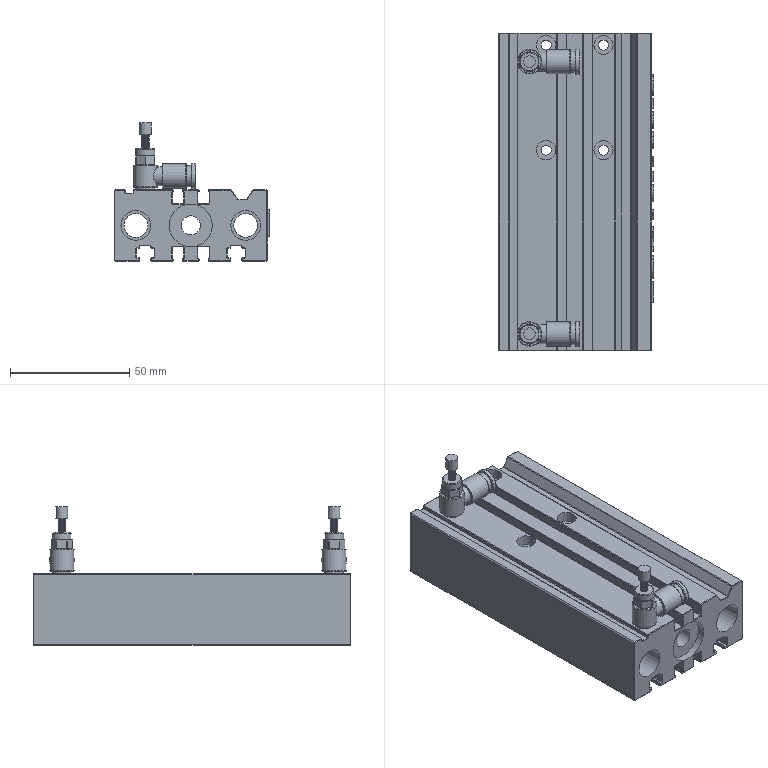Part | STEP file | Tube necking machine_id346_x_t | 1 solid | 722 faces | box 65 x 133 x 58 mm | volume 191780 mm3 | plane 589 | other 74 | cylinder 39 | torus 12 | spline 8 | commonest cylinder face diameters 8 x11 4.2 x4 10.3 x4 15 x3 2.5 x2 3 x2